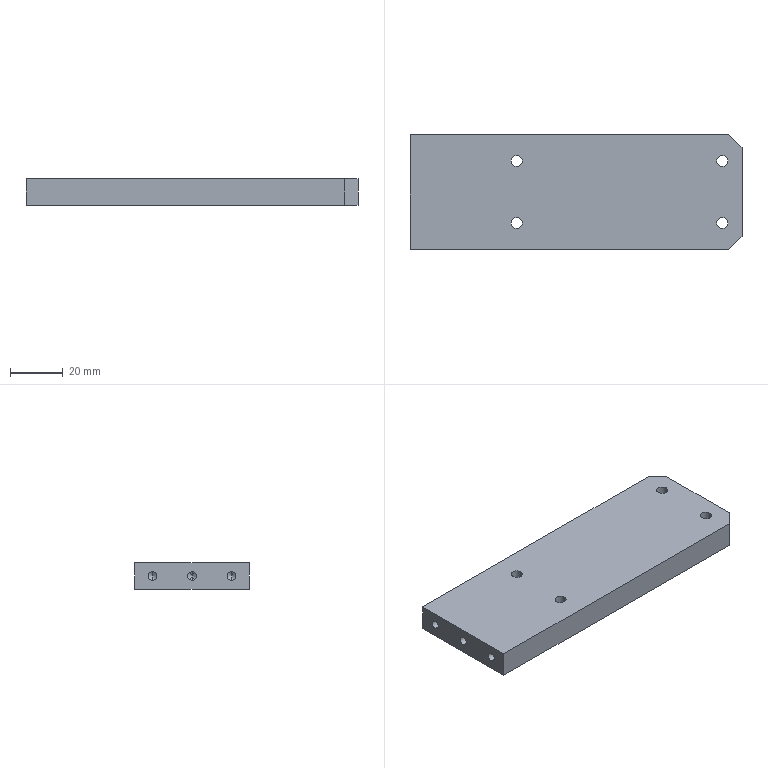Part | SolidWorks | features HoleWzd 2, Chamfer 1, Extrusion 1 | 1 solid | 28 faces | box 126 x 43.6 x 10 mm | volume 53864 mm3 | cylinder 14 | plane 8 | cone 6 | commonest cylinder face diameters 4.2 x8 3.3 x6
STEP:
#1=CARTESIAN_POINT('',(42.6,33.55,0.));
#2=VERTEX_POINT('',#1);
#3=CARTESIAN_POINT('',(38.4,33.55,0.));
#4=VERTEX_POINT('',#3);
#5=CARTESIAN_POINT('',(40.5,33.55,0.));
#6=DIRECTION('',(0.,0.,-1.));
#7=DIRECTION('',(-1.,0.,0.));
#8=AXIS2_PLACEMENT_3D('',#5,#6,#7);
#9=CIRCLE('',#8,2.1);
#10=EDGE_CURVE('',#2,#4,#9,.T.);
#11=ORIENTED_EDGE('',*,*,#10,.F.);
#12=CARTESIAN_POINT('',(42.6,33.55,-10.));
#13=VERTEX_POINT('',#12);
#14=CARTESIAN_POINT('',(42.6,33.55,-10.));
#15=DIRECTION('',(0.,0.,-1.));
#16=VECTOR('',#15,1000.);
#17=LINE('',#14,#16);
#18=EDGE_CURVE('',#2,#13,#17,.T.);
#19=ORIENTED_EDGE('',*,*,#18,.T.);
#20=CARTESIAN_POINT('',(38.4,33.55,-10.));
#21=VERTEX_POINT('',#20);
#22=CARTESIAN_POINT('',(40.5,33.55,-10.));
#23=DIRECTION('',(0.,0.,-1.));
#24=DIRECTION('',(-1.,0.,0.));
#25=AXIS2_PLACEMENT_3D('',#22,#23,#24);
#26=CIRCLE('',#25,2.1);
#27=EDGE_CURVE('',#13,#21,#26,.T.);
#28=ORIENTED_EDGE('',*,*,#27,.T.);
#29=CARTESIAN_POINT('',(38.4,33.55,-10.));
#30=DIRECTION('',(0.,0.,-1.));
#31=VECTOR('',#30,1000.);
#32=LINE('',#29,#31);
#33=EDGE_CURVE('',#4,#21,#32,.T.);
#34=ORIENTED_EDGE('',*,*,#33,.F.);
#35=EDGE_LOOP('',(#11,#19,#28,#34));
#36=FACE_OUTER_BOUND('',#35,.T.);
#37=CARTESIAN_POINT('',(40.5,33.55,-10.));
#38=DIRECTION('',(0.,0.,-1.));
#39=DIRECTION('',(-1.,0.,0.));
#40=AXIS2_PLACEMENT_3D('',#37,#38,#39);
#41=CYLINDRICAL_SURFACE('',#40,2.1);
#42=ADVANCED_FACE('',(#36),#41,.F.);
#43=CARTESIAN_POINT('',(42.6,10.05,0.));
#44=VERTEX_POINT('',#43);
#45=CARTESIAN_POINT('',(38.4,10.05,0.));
#46=VERTEX_POINT('',#45);
#47=CARTESIAN_POINT('',(40.5,10.05,0.));
#48=DIRECTION('',(0.,0.,-1.));
#49=DIRECTION('',(-1.,0.,0.));
#50=AXIS2_PLACEMENT_3D('',#47,#48,#49);
#51=CIRCLE('',#50,2.1);
#52=EDGE_CURVE('',#44,#46,#51,.T.);
#53=ORIENTED_EDGE('',*,*,#52,.F.);
#54=CARTESIAN_POINT('',(42.6,10.05,-10.));
#55=VERTEX_POINT('',#54);
#56=CARTESIAN_POINT('',(42.6,10.05,-10.));
#57=DIRECTION('',(0.,0.,-1.));
#58=VECTOR('',#57,1000.);
#59=LINE('',#56,#58);
#60=EDGE_CURVE('',#44,#55,#59,.T.);
#61=ORIENTED_EDGE('',*,*,#60,.T.);
#62=CARTESIAN_POINT('',(38.4,10.05,-10.));
#63=VERTEX_POINT('',#62);
#64=CARTESIAN_POINT('',(40.5,10.05,-10.));
#65=DIRECTION('',(0.,0.,-1.));
#66=DIRECTION('',(-1.,0.,0.));
#67=AXIS2_PLACEMENT_3D('',#64,#65,#66);
#68=CIRCLE('',#67,2.1);
#69=EDGE_CURVE('',#55,#63,#68,.T.);
#70=ORIENTED_EDGE('',*,*,#69,.T.);
#71=CARTESIAN_POINT('',(38.4,10.05,-10.));
#72=DIRECTION('',(0.,0.,-1.));
#73=VECTOR('',#72,1000.);
#74=LINE('',#71,#73);
#75=EDGE_CURVE('',#46,#63,#74,.T.);
#76=ORIENTED_EDGE('',*,*,#75,.F.);
#77=EDGE_LOOP('',(#53,#61,#70,#76));
#78=FACE_OUTER_BOUND('',#77,.T.);
#79=CARTESIAN_POINT('',(40.5,10.05,-10.));
#80=DIRECTION('',(0.,0.,-1.));
#81=DIRECTION('',(-1.,0.,0.));
#82=AXIS2_PLACEMENT_3D('',#79,#80,#81);
#83=CYLINDRICAL_SURFACE('',#82,2.1);
#84=ADVANCED_FACE('',(#78),#83,.F.);
#85=CARTESIAN_POINT('',(120.6,33.55,0.));
#86=VERTEX_POINT('',#85);
#87=CARTESIAN_POINT('',(116.4,33.55,0.));
#88=VERTEX_POINT('',#87);
#89=CARTESIAN_POINT('',(118.5,33.55,0.));
#90=DIRECTION('',(0.,0.,-1.));
#91=DIRECTION('',(-1.,0.,0.));
#92=AXIS2_PLACEMENT_3D('',#89,#90,#91);
#93=CIRCLE('',#92,2.1);
#94=EDGE_CURVE('',#86,#88,#93,.T.);
#95=ORIENTED_EDGE('',*,*,#94,.F.);
#96=CARTESIAN_POINT('',(120.6,33.55,-10.));
#97=VERTEX_POINT('',#96);
#98=CARTESIAN_POINT('',(120.6,33.55,-10.));
#99=DIRECTION('',(0.,0.,-1.));
#100=VECTOR('',#99,1000.);
#101=LINE('',#98,#100);
#102=EDGE_CURVE('',#86,#97,#101,.T.);
#103=ORIENTED_EDGE('',*,*,#102,.T.);
#104=CARTESIAN_POINT('',(116.4,33.55,-10.));
#105=VERTEX_POINT('',#104);
#106=CARTESIAN_POINT('',(118.5,33.55,-10.));
#107=DIRECTION('',(0.,0.,-1.));
#108=DIRECTION('',(-1.,0.,0.));
#109=AXIS2_PLACEMENT_3D('',#106,#107,#108);
#110=CIRCLE('',#109,2.1);
#111=EDGE_CURVE('',#97,#105,#110,.T.);
#112=ORIENTED_EDGE('',*,*,#111,.T.);
#113=CARTESIAN_POINT('',(116.4,33.55,-10.));
#114=DIRECTION('',(0.,0.,-1.));
#115=VECTOR('',#114,1000.);
#116=LINE('',#113,#115);
#117=EDGE_CURVE('',#88,#105,#116,.T.);
#118=ORIENTED_EDGE('',*,*,#117,.F.);
#119=EDGE_LOOP('',(#95,#103,#112,#118));
#120=FACE_OUTER_BOUND('',#119,.T.);
#121=CARTESIAN_POINT('',(118.5,33.55,-10.));
#122=DIRECTION('',(0.,0.,-1.));
#123=DIRECTION('',(-1.,0.,0.));
#124=AXIS2_PLACEMENT_3D('',#121,#122,#123);
#125=CYLINDRICAL_SURFACE('',#124,2.1);
#126=ADVANCED_FACE('',(#120),#125,.F.);
#127=CARTESIAN_POINT('',(120.6,10.05,0.));
#128=VERTEX_POINT('',#127);
#129=CARTESIAN_POINT('',(116.4,10.05,0.));
#130=VERTEX_POINT('',#129);
#131=CARTESIAN_POINT('',(118.5,10.05,0.));
#132=DIRECTION('',(0.,0.,-1.));
#133=DIRECTION('',(-1.,0.,0.));
#134=AXIS2_PLACEMENT_3D('',#131,#132,#133);
#135=CIRCLE('',#134,2.1);
#136=EDGE_CURVE('',#128,#130,#135,.T.);
#137=ORIENTED_EDGE('',*,*,#136,.F.);
#138=CARTESIAN_POINT('',(120.6,10.05,-10.));
#139=VERTEX_POINT('',#138);
#140=CARTESIAN_POINT('',(120.6,10.05,-10.));
#141=DIRECTION('',(0.,0.,-1.));
#142=VECTOR('',#141,1000.);
#143=LINE('',#140,#142);
#144=EDGE_CURVE('',#128,#139,#143,.T.);
#145=ORIENTED_EDGE('',*,*,#144,.T.);
#146=CARTESIAN_POINT('',(116.4,10.05,-10.));
#147=VERTEX_POINT('',#146);
#148=CARTESIAN_POINT('',(118.5,10.05,-10.));
#149=DIRECTION('',(0.,0.,-1.));
#150=DIRECTION('',(-1.,0.,0.));
#151=AXIS2_PLACEMENT_3D('',#148,#149,#150);
#152=CIRCLE('',#151,2.1);
#153=EDGE_CURVE('',#139,#147,#152,.T.);
#154=ORIENTED_EDGE('',*,*,#153,.T.);
#155=CARTESIAN_POINT('',(116.4,10.05,-10.));
#156=DIRECTION('',(0.,0.,-1.));
#157=VECTOR('',#156,1000.);
#158=LINE('',#155,#157);
#159=EDGE_CURVE('',#130,#147,#158,.T.);
#160=ORIENTED_EDGE('',*,*,#159,.F.);
#161=EDGE_LOOP('',(#137,#145,#154,#160));
#162=FACE_OUTER_BOUND('',#161,.T.);
#163=CARTESIAN_POINT('',(118.5,10.05,-10.));
#164=DIRECTION('',(0.,0.,-1.));
#165=DIRECTION('',(-1.,0.,0.));
#166=AXIS2_PLACEMENT_3D('',#163,#164,#165);
#167=CYLINDRICAL_SURFACE('',#166,2.1);
#168=ADVANCED_FACE('',(#162),#167,.F.);
#169=CARTESIAN_POINT('',(10.1,36.8,-6.65));
#170=VERTEX_POINT('',#169);
#171=CARTESIAN_POINT('',(10.1,36.8,-3.35));
#172=VERTEX_POINT('',#171);
#173=CARTESIAN_POINT('',(10.1,36.8,-5.));
#174=DIRECTION('',(-1.,0.,0.));
#175=DIRECTION('',(0.,0.,1.));
#176=AXIS2_PLACEMENT_3D('',#173,#174,#175);
#177=CIRCLE('',#176,1.65);
#178=EDGE_CURVE('',#170,#172,#177,.T.);
#179=ORIENTED_EDGE('',*,*,#178,.F.);
#180=CARTESIAN_POINT('',(0.,36.8,-6.65));
#181=VERTEX_POINT('',#180);
#182=CARTESIAN_POINT('',(0.,36.8,-6.65));
#183=DIRECTION('',(-1.,0.,0.));
#184=VECTOR('',#183,1000.);
#185=LINE('',#182,#184);
#186=EDGE_CURVE('',#170,#181,#185,.T.);
#187=ORIENTED_EDGE('',*,*,#186,.T.);
#188=CARTESIAN_POINT('',(0.,36.8,-3.35));
#189=VERTEX_POINT('',#188);
#190=CARTESIAN_POINT('',(0.,36.8,-5.));
#191=DIRECTION('',(-1.,0.,0.));
#192=DIRECTION('',(0.,0.,1.));
#193=AXIS2_PLACEMENT_3D('',#190,#191,#192);
#194=CIRCLE('',#193,1.65);
#195=EDGE_CURVE('',#181,#189,#194,.T.);
#196=ORIENTED_EDGE('',*,*,#195,.T.);
#197=CARTESIAN_POINT('',(0.,36.8,-3.35));
#198=DIRECTION('',(-1.,0.,0.));
#199=VECTOR('',#198,1000.);
#200=LINE('',#197,#199);
#201=EDGE_CURVE('',#172,#189,#200,.T.);
#202=ORIENTED_EDGE('',*,*,#201,.F.);
#203=EDGE_LOOP('',(#179,#187,#196,#202));
#204=FACE_OUTER_BOUND('',#203,.T.);
#205=CARTESIAN_POINT('',(0.,36.8,-5.));
#206=DIRECTION('',(-1.,0.,0.));
#207=DIRECTION('',(0.,0.,1.));
#208=AXIS2_PLACEMENT_3D('',#205,#206,#207);
#209=CYLINDRICAL_SURFACE('',#208,1.65);
#210=ADVANCED_FACE('',(#204),#209,.F.);
#211=CARTESIAN_POINT('',(11.091,36.8,-5.));
#212=VERTEX_POINT('',#211);
#213=CARTESIAN_POINT('',(10.1,36.8,-3.35));
#214=DIRECTION('',(-0.515,0.,0.8572));
#215=VECTOR('',#214,1000.);
#216=LINE('',#213,#215);
#217=EDGE_CURVE('',#212,#172,#216,.T.);
#218=ORIENTED_EDGE('',*,*,#217,.F.);
#219=CARTESIAN_POINT('',(10.1,36.8,-6.65));
#220=DIRECTION('',(-0.515,0.,-0.8572));
#221=VECTOR('',#220,1000.);
#222=LINE('',#219,#221);
#223=EDGE_CURVE('',#212,#170,#222,.T.);
#224=ORIENTED_EDGE('',*,*,#223,.T.);
#225=ORIENTED_EDGE('',*,*,#178,.T.);
#226=EDGE_LOOP('',(#218,#224,#225));
#227=FACE_OUTER_BOUND('',#226,.T.);
#228=CARTESIAN_POINT('',(10.1,36.8,-5.));
#229=DIRECTION('',(-1.,0.,0.));
#230=DIRECTION('',(0.,0.,1.));
#231=AXIS2_PLACEMENT_3D('',#228,#229,#230);
#232=CONICAL_SURFACE('',#231,1.65,1.03);
#233=ADVANCED_FACE('',(#227),#232,.F.);
#234=CARTESIAN_POINT('',(10.1,21.783,-6.65));
#235=VERTEX_POINT('',#234);
#236=CARTESIAN_POINT('',(10.1,21.783,-3.35));
#237=VERTEX_POINT('',#236);
#238=CARTESIAN_POINT('',(10.1,21.783,-5.));
#239=DIRECTION('',(-1.,0.,0.));
#240=DIRECTION('',(0.,0.,1.));
#241=AXIS2_PLACEMENT_3D('',#238,#239,#240);
#242=CIRCLE('',#241,1.65);
#243=EDGE_CURVE('',#235,#237,#242,.T.);
#244=ORIENTED_EDGE('',*,*,#243,.F.);
#245=CARTESIAN_POINT('',(0.,21.783,-6.65));
#246=VERTEX_POINT('',#245);
#247=CARTESIAN_POINT('',(0.,21.783,-6.65));
#248=DIRECTION('',(-1.,0.,0.));
#249=VECTOR('',#248,1000.);
#250=LINE('',#247,#249);
#251=EDGE_CURVE('',#235,#246,#250,.T.);
#252=ORIENTED_EDGE('',*,*,#251,.T.);
#253=CARTESIAN_POINT('',(0.,21.783,-3.35));
#254=VERTEX_POINT('',#253);
#255=CARTESIAN_POINT('',(0.,21.783,-5.));
#256=DIRECTION('',(-1.,0.,0.));
#257=DIRECTION('',(0.,0.,1.));
#258=AXIS2_PLACEMENT_3D('',#255,#256,#257);
#259=CIRCLE('',#258,1.65);
#260=EDGE_CURVE('',#246,#254,#259,.T.);
#261=ORIENTED_EDGE('',*,*,#260,.T.);
#262=CARTESIAN_POINT('',(0.,21.783,-3.35));
#263=DIRECTION('',(-1.,0.,0.));
#264=VECTOR('',#263,1000.);
#265=LINE('',#262,#264);
#266=EDGE_CURVE('',#237,#254,#265,.T.);
#267=ORIENTED_EDGE('',*,*,#266,.F.);
#268=EDGE_LOOP('',(#244,#252,#261,#267));
#269=FACE_OUTER_BOUND('',#268,.T.);
#270=CARTESIAN_POINT('',(0.,21.783,-5.));
#271=DIRECTION('',(-1.,0.,0.));
#272=DIRECTION('',(0.,0.,1.));
#273=AXIS2_PLACEMENT_3D('',#270,#271,#272);
#274=CYLINDRICAL_SURFACE('',#273,1.65);
#275=ADVANCED_FACE('',(#269),#274,.F.);
#276=CARTESIAN_POINT('',(11.091,21.783,-5.));
#277=VERTEX_POINT('',#276);
#278=CARTESIAN_POINT('',(10.1,21.783,-3.35));
#279=DIRECTION('',(-0.515,0.,0.8572));
#280=VECTOR('',#279,1000.);
#281=LINE('',#278,#280);
#282=EDGE_CURVE('',#277,#237,#281,.T.);
#283=ORIENTED_EDGE('',*,*,#282,.F.);
#284=CARTESIAN_POINT('',(10.1,21.783,-6.65));
#285=DIRECTION('',(-0.515,0.,-0.8572));
#286=VECTOR('',#285,1000.);
#287=LINE('',#284,#286);
#288=EDGE_CURVE('',#277,#235,#287,.T.);
#289=ORIENTED_EDGE('',*,*,#288,.T.);
#290=ORIENTED_EDGE('',*,*,#243,.T.);
#291=EDGE_LOOP('',(#283,#289,#290));
#292=FACE_OUTER_BOUND('',#291,.T.);
#293=CARTESIAN_POINT('',(10.1,21.783,-5.));
#294=DIRECTION('',(-1.,0.,0.));
#295=DIRECTION('',(0.,0.,1.));
#296=AXIS2_PLACEMENT_3D('',#293,#294,#295);
#297=CONICAL_SURFACE('',#296,1.65,1.03);
#298=ADVANCED_FACE('',(#292),#297,.F.);
#299=CARTESIAN_POINT('',(10.1,6.8,-6.65));
#300=VERTEX_POINT('',#299);
#301=CARTESIAN_POINT('',(10.1,6.8,-3.35));
#302=VERTEX_POINT('',#301);
#303=CARTESIAN_POINT('',(10.1,6.8,-5.));
#304=DIRECTION('',(-1.,0.,0.));
#305=DIRECTION('',(0.,0.,1.));
#306=AXIS2_PLACEMENT_3D('',#303,#304,#305);
#307=CIRCLE('',#306,1.65);
#308=EDGE_CURVE('',#300,#302,#307,.T.);
#309=ORIENTED_EDGE('',*,*,#308,.F.);
#310=CARTESIAN_POINT('',(0.,6.8,-6.65));
#311=VERTEX_POINT('',#310);
#312=CARTESIAN_POINT('',(0.,6.8,-6.65));
#313=DIRECTION('',(-1.,0.,0.));
#314=VECTOR('',#313,1000.);
#315=LINE('',#312,#314);
#316=EDGE_CURVE('',#300,#311,#315,.T.);
#317=ORIENTED_EDGE('',*,*,#316,.T.);
#318=CARTESIAN_POINT('',(0.,6.8,-3.35));
#319=VERTEX_POINT('',#318);
#320=CARTESIAN_POINT('',(0.,6.8,-5.));
#321=DIRECTION('',(-1.,0.,0.));
#322=DIRECTION('',(0.,0.,1.));
#323=AXIS2_PLACEMENT_3D('',#320,#321,#322);
#324=CIRCLE('',#323,1.65);
#325=EDGE_CURVE('',#311,#319,#324,.T.);
#326=ORIENTED_EDGE('',*,*,#325,.T.);
#327=CARTESIAN_POINT('',(0.,6.8,-3.35));
#328=DIRECTION('',(-1.,0.,0.));
#329=VECTOR('',#328,1000.);
#330=LINE('',#327,#329);
#331=EDGE_CURVE('',#302,#319,#330,.T.);
#332=ORIENTED_EDGE('',*,*,#331,.F.);
#333=EDGE_LOOP('',(#309,#317,#326,#332));
#334=FACE_OUTER_BOUND('',#333,.T.);
#335=CARTESIAN_POINT('',(0.,6.8,-5.));
#336=DIRECTION('',(-1.,0.,0.));
#337=DIRECTION('',(0.,0.,1.));
#338=AXIS2_PLACEMENT_3D('',#335,#336,#337);
#339=CYLINDRICAL_SURFACE('',#338,1.65);
#340=ADVANCED_FACE('',(#334),#339,.F.);
#341=CARTESIAN_POINT('',(11.091,6.8,-5.));
#342=VERTEX_POINT('',#341);
#343=CARTESIAN_POINT('',(10.1,6.8,-3.35));
#344=DIRECTION('',(-0.515,0.,0.8572));
#345=VECTOR('',#344,1000.);
#346=LINE('',#343,#345);
#347=EDGE_CURVE('',#342,#302,#346,.T.);
#348=ORIENTED_EDGE('',*,*,#347,.F.);
#349=CARTESIAN_POINT('',(10.1,6.8,-6.65));
#350=DIRECTION('',(-0.515,0.,-0.8572));
#351=VECTOR('',#350,1000.);
#352=LINE('',#349,#351);
#353=EDGE_CURVE('',#342,#300,#352,.T.);
#354=ORIENTED_EDGE('',*,*,#353,.T.);
#355=ORIENTED_EDGE('',*,*,#308,.T.);
#356=EDGE_LOOP('',(#348,#354,#355));
#357=FACE_OUTER_BOUND('',#356,.T.);
#358=CARTESIAN_POINT('',(10.1,6.8,-5.));
#359=DIRECTION('',(-1.,0.,0.));
#360=DIRECTION('',(0.,0.,1.));
#361=AXIS2_PLACEMENT_3D('',#358,#359,#360);
#362=CONICAL_SURFACE('',#361,1.65,1.03);
#363=ADVANCED_FACE('',(#357),#362,.F.);
#364=CARTESIAN_POINT('',(0.,36.8,-5.));
#365=DIRECTION('',(-1.,0.,0.));
#366=DIRECTION('',(0.,0.,1.));
#367=AXIS2_PLACEMENT_3D('',#364,#365,#366);
#368=CIRCLE('',#367,1.65);
#369=EDGE_CURVE('',#189,#181,#368,.T.);
#370=ORIENTED_EDGE('',*,*,#369,.F.);
#371=ORIENTED_EDGE('',*,*,#195,.F.);
#372=EDGE_LOOP('',(#370,#371));
#373=FACE_BOUND('',#372,.T.);
#374=CARTESIAN_POINT('',(0.,21.783,-5.));
#375=DIRECTION('',(-1.,0.,0.));
#376=DIRECTION('',(0.,0.,1.));
#377=AXIS2_PLACEMENT_3D('',#374,#375,#376);
#378=CIRCLE('',#377,1.65);
#379=EDGE_CURVE('',#254,#246,#378,.T.);
#380=ORIENTED_EDGE('',*,*,#379,.F.);
#381=ORIENTED_EDGE('',*,*,#260,.F.);
#382=EDGE_LOOP('',(#380,#381));
#383=FACE_BOUND('',#382,.T.);
#384=CARTESIAN_POINT('',(0.,6.8,-5.));
#385=DIRECTION('',(-1.,0.,0.));
#386=DIRECTION('',(0.,0.,1.));
#387=AXIS2_PLACEMENT_3D('',#384,#385,#386);
#388=CIRCLE('',#387,1.65);
#389=EDGE_CURVE('',#319,#311,#388,.T.);
#390=ORIENTED_EDGE('',*,*,#389,.F.);
#391=ORIENTED_EDGE('',*,*,#325,.F.);
#392=EDGE_LOOP('',(#390,#391));
#393=FACE_BOUND('',#392,.T.);
#394=CARTESIAN_POINT('',(0.,0.,-10.));
#395=VERTEX_POINT('',#394);
#396=CARTESIAN_POINT('',(0.,0.,0.));
#397=VERTEX_POINT('',#396);
#398=CARTESIAN_POINT('',(0.,0.,0.));
#399=DIRECTION('',(0.,0.,1.));
#400=VECTOR('',#399,1000.);
#401=LINE('',#398,#400);
#402=EDGE_CURVE('',#395,#397,#401,.T.);
#403=ORIENTED_EDGE('',*,*,#402,.T.);
#404=CARTESIAN_POINT('',(0.,43.6,0.));
#405=VERTEX_POINT('',#404);
#406=CARTESIAN_POINT('',(0.,43.6,0.));
#407=DIRECTION('',(0.,-1.,0.));
#408=VECTOR('',#407,1000.);
#409=LINE('',#406,#408);
#410=EDGE_CURVE('',#405,#397,#409,.T.);
#411=ORIENTED_EDGE('',*,*,#410,.F.);
#412=CARTESIAN_POINT('',(0.,43.6,-10.));
#413=VERTEX_POINT('',#412);
#414=CARTESIAN_POINT('',(0.,43.6,0.));
#415=DIRECTION('',(0.,0.,1.));
#416=VECTOR('',#415,1000.);
#417=LINE('',#414,#416);
#418=EDGE_CURVE('',#413,#405,#417,.T.);
#419=ORIENTED_EDGE('',*,*,#418,.F.);
#420=CARTESIAN_POINT('',(0.,43.6,-10.));
#421=DIRECTION('',(0.,-1.,0.));
#422=VECTOR('',#421,1000.);
#423=LINE('',#420,#422);
#424=EDGE_CURVE('',#413,#395,#423,.T.);
#425=ORIENTED_EDGE('',*,*,#424,.T.);
#426=EDGE_LOOP('',(#403,#411,#419,#425));
#427=FACE_OUTER_BOUND('',#426,.T.);
#428=CARTESIAN_POINT('',(0.,43.6,0.));
#429=DIRECTION('',(1.,0.,0.));
#430=DIRECTION('',(0.,0.,-1.));
#431=AXIS2_PLACEMENT_3D('',#428,#429,#430);
#432=PLANE('',#431);
#433=ADVANCED_FACE('',(#373,#383,#393,#427),#432,.F.);
#434=CARTESIAN_POINT('',(40.5,33.55,0.));
#435=DIRECTION('',(0.,0.,-1.));
#436=DIRECTION('',(-1.,0.,0.));
#437=AXIS2_PLACEMENT_3D('',#434,#435,#436);
#438=CIRCLE('',#437,2.1);
#439=EDGE_CURVE('',#4,#2,#438,.T.);
#440=ORIENTED_EDGE('',*,*,#439,.T.);
#441=ORIENTED_EDGE('',*,*,#10,.T.);
#442=EDGE_LOOP('',(#440,#441));
#443=FACE_BOUND('',#442,.T.);
#444=CARTESIAN_POINT('',(40.5,10.05,0.));
#445=DIRECTION('',(0.,0.,-1.));
#446=DIRECTION('',(-1.,0.,0.));
#447=AXIS2_PLACEMENT_3D('',#444,#445,#446);
#448=CIRCLE('',#447,2.1);
#449=EDGE_CURVE('',#46,#44,#448,.T.);
#450=ORIENTED_EDGE('',*,*,#449,.T.);
#451=ORIENTED_EDGE('',*,*,#52,.T.);
#452=EDGE_LOOP('',(#450,#451));
#453=FACE_BOUND('',#452,.T.);
#454=CARTESIAN_POINT('',(118.5,33.55,0.));
#455=DIRECTION('',(0.,0.,-1.));
#456=DIRECTION('',(-1.,0.,0.));
#457=AXIS2_PLACEMENT_3D('',#454,#455,#456);
#458=CIRCLE('',#457,2.1);
#459=EDGE_CURVE('',#88,#86,#458,.T.);
#460=ORIENTED_EDGE('',*,*,#459,.T.);
#461=ORIENTED_EDGE('',*,*,#94,.T.);
#462=EDGE_LOOP('',(#460,#461));
#463=FACE_BOUND('',#462,.T.);
#464=CARTESIAN_POINT('',(118.5,10.05,0.));
#465=DIRECTION('',(0.,0.,-1.));
#466=DIRECTION('',(-1.,0.,0.));
#467=AXIS2_PLACEMENT_3D('',#464,#465,#466);
#468=CIRCLE('',#467,2.1);
#469=EDGE_CURVE('',#130,#128,#468,.T.);
#470=ORIENTED_EDGE('',*,*,#469,.T.);
#471=ORIENTED_EDGE('',*,*,#136,.T.);
#472=EDGE_LOOP('',(#470,#471));
#473=FACE_BOUND('',#472,.T.);
#474=CARTESIAN_POINT('',(121.,0.,0.));
#475=VERTEX_POINT('',#474);
#476=CARTESIAN_POINT('',(0.,0.,0.));
#477=DIRECTION('',(1.,0.,0.));
#478=VECTOR('',#477,1000.);
#479=LINE('',#476,#478);
#480=EDGE_CURVE('',#397,#475,#479,.T.);
#481=ORIENTED_EDGE('',*,*,#480,.T.);
#482=CARTESIAN_POINT('',(126.,5.,0.));
#483=VERTEX_POINT('',#482);
#484=CARTESIAN_POINT('',(126.,5.,0.));
#485=DIRECTION('',(0.7071,0.7071,0.));
#486=VECTOR('',#485,1000.);
#487=LINE('',#484,#486);
#488=EDGE_CURVE('',#475,#483,#487,.T.);
#489=ORIENTED_EDGE('',*,*,#488,.T.);
#490=CARTESIAN_POINT('',(126.,38.6,0.));
#491=VERTEX_POINT('',#490);
#492=CARTESIAN_POINT('',(126.,43.6,0.));
#493=DIRECTION('',(0.,-1.,0.));
#494=VECTOR('',#493,1000.);
#495=LINE('',#492,#494);
#496=EDGE_CURVE('',#491,#483,#495,.T.);
#497=ORIENTED_EDGE('',*,*,#496,.F.);
#498=CARTESIAN_POINT('',(121.,43.6,0.));
#499=VERTEX_POINT('',#498);
#500=CARTESIAN_POINT('',(121.,43.6,0.));
#501=DIRECTION('',(-0.7071,0.7071,0.));
#502=VECTOR('',#501,1000.);
#503=LINE('',#500,#502);
#504=EDGE_CURVE('',#491,#499,#503,.T.);
#505=ORIENTED_EDGE('',*,*,#504,.T.);
#506=CARTESIAN_POINT('',(0.,43.6,0.));
#507=DIRECTION('',(1.,0.,0.));
#508=VECTOR('',#507,1000.);
#509=LINE('',#506,#508);
#510=EDGE_CURVE('',#405,#499,#509,.T.);
#511=ORIENTED_EDGE('',*,*,#510,.F.);
#512=ORIENTED_EDGE('',*,*,#410,.T.);
#513=EDGE_LOOP('',(#481,#489,#497,#505,#511,#512));
#514=FACE_OUTER_BOUND('',#513,.T.);
#515=CARTESIAN_POINT('',(0.,43.6,0.));
#516=DIRECTION('',(0.,0.,-1.));
#517=DIRECTION('',(-1.,0.,0.));
#518=AXIS2_PLACEMENT_3D('',#515,#516,#517);
#519=PLANE('',#518);
#520=ADVANCED_FACE('',(#443,#453,#463,#473,#514),#519,.F.);
#521=ORIENTED_EDGE('',*,*,#496,.T.);
#522=CARTESIAN_POINT('',(126.,5.,-10.));
#523=VERTEX_POINT('',#522);
#524=CARTESIAN_POINT('',(126.,5.,-10.));
#525=DIRECTION('',(0.,0.,-1.));
#526=VECTOR('',#525,1000.);
#527=LINE('',#524,#526);
#528=EDGE_CURVE('',#483,#523,#527,.T.);
#529=ORIENTED_EDGE('',*,*,#528,.T.);
#530=CARTESIAN_POINT('',(126.,38.6,-10.));
#531=VERTEX_POINT('',#530);
#532=CARTESIAN_POINT('',(126.,43.6,-10.));
#533=DIRECTION('',(0.,-1.,0.));
#534=VECTOR('',#533,1000.);
#535=LINE('',#532,#534);
#536=EDGE_CURVE('',#531,#523,#535,.T.);
#537=ORIENTED_EDGE('',*,*,#536,.F.);
#538=CARTESIAN_POINT('',(126.,38.6,0.));
#539=DIRECTION('',(0.,0.,1.));
#540=VECTOR('',#539,1000.);
#541=LINE('',#538,#540);
#542=EDGE_CURVE('',#531,#491,#541,.T.);
#543=ORIENTED_EDGE('',*,*,#542,.T.);
#544=EDGE_LOOP('',(#521,#529,#537,#543));
#545=FACE_OUTER_BOUND('',#544,.T.);
#546=CARTESIAN_POINT('',(126.,43.6,0.));
#547=DIRECTION('',(-1.,0.,0.));
#548=DIRECTION('',(0.,0.,1.));
#549=AXIS2_PLACEMENT_3D('',#546,#547,#548);
#550=PLANE('',#549);
#551=ADVANCED_FACE('',(#545),#550,.F.);
#552=CARTESIAN_POINT('',(40.5,33.55,-10.));
#553=DIRECTION('',(0.,0.,-1.));
#554=DIRECTION('',(-1.,0.,0.));
#555=AXIS2_PLACEMENT_3D('',#552,#553,#554);
#556=CIRCLE('',#555,2.1);
#557=EDGE_CURVE('',#21,#13,#556,.T.);
#558=ORIENTED_EDGE('',*,*,#557,.F.);
#559=ORIENTED_EDGE('',*,*,#27,.F.);
#560=EDGE_LOOP('',(#558,#559));
#561=FACE_BOUND('',#560,.T.);
#562=CARTESIAN_POINT('',(40.5,10.05,-10.));
#563=DIRECTION('',(0.,0.,-1.));
#564=DIRECTION('',(-1.,0.,0.));
#565=AXIS2_PLACEMENT_3D('',#562,#563,#564);
#566=CIRCLE('',#565,2.1);
#567=EDGE_CURVE('',#63,#55,#566,.T.);
#568=ORIENTED_EDGE('',*,*,#567,.F.);
#569=ORIENTED_EDGE('',*,*,#69,.F.);
#570=EDGE_LOOP('',(#568,#569));
#571=FACE_BOUND('',#570,.T.);
#572=CARTESIAN_POINT('',(118.5,33.55,-10.));
#573=DIRECTION('',(0.,0.,-1.));
#574=DIRECTION('',(-1.,0.,0.));
#575=AXIS2_PLACEMENT_3D('',#572,#573,#574);
#576=CIRCLE('',#575,2.1);
#577=EDGE_CURVE('',#105,#97,#576,.T.);
#578=ORIENTED_EDGE('',*,*,#577,.F.);
#579=ORIENTED_EDGE('',*,*,#111,.F.);
#580=EDGE_LOOP('',(#578,#579));
#581=FACE_BOUND('',#580,.T.);
#582=CARTESIAN_POINT('',(118.5,10.05,-10.));
#583=DIRECTION('',(0.,0.,-1.));
#584=DIRECTION('',(-1.,0.,0.));
#585=AXIS2_PLACEMENT_3D('',#582,#583,#584);
#586=CIRCLE('',#585,2.1);
#587=EDGE_CURVE('',#147,#139,#586,.T.);
#588=ORIENTED_EDGE('',*,*,#587,.F.);
#589=ORIENTED_EDGE('',*,*,#153,.F.);
#590=EDGE_LOOP('',(#588,#589));
#591=FACE_BOUND('',#590,.T.);
#592=ORIENTED_EDGE('',*,*,#536,.T.);
#593=CARTESIAN_POINT('',(121.,0.,-10.));
#594=VERTEX_POINT('',#593);
#595=CARTESIAN_POINT('',(126.,5.,-10.));
#596=DIRECTION('',(-0.7071,-0.7071,0.));
#597=VECTOR('',#596,1000.);
#598=LINE('',#595,#597);
#599=EDGE_CURVE('',#523,#594,#598,.T.);
#600=ORIENTED_EDGE('',*,*,#599,.T.);
#601=CARTESIAN_POINT('',(0.,0.,-10.));
#602=DIRECTION('',(-1.,0.,0.));
#603=VECTOR('',#602,1000.);
#604=LINE('',#601,#603);
#605=EDGE_CURVE('',#594,#395,#604,.T.);
#606=ORIENTED_EDGE('',*,*,#605,.T.);
#607=ORIENTED_EDGE('',*,*,#424,.F.);
#608=CARTESIAN_POINT('',(121.,43.6,-10.));
#609=VERTEX_POINT('',#608);
#610=CARTESIAN_POINT('',(0.,43.6,-10.));
#611=DIRECTION('',(-1.,0.,0.));
#612=VECTOR('',#611,1000.);
#613=LINE('',#610,#612);
#614=EDGE_CURVE('',#609,#413,#613,.T.);
#615=ORIENTED_EDGE('',*,*,#614,.F.);
#616=CARTESIAN_POINT('',(121.,43.6,-10.));
#617=DIRECTION('',(0.7071,-0.7071,0.));
#618=VECTOR('',#617,1000.);
#619=LINE('',#616,#618);
#620=EDGE_CURVE('',#609,#531,#619,.T.);
#621=ORIENTED_EDGE('',*,*,#620,.T.);
#622=EDGE_LOOP('',(#592,#600,#606,#607,#615,#621));
#623=FACE_OUTER_BOUND('',#622,.T.);
#624=CARTESIAN_POINT('',(0.,43.6,-10.));
#625=DIRECTION('',(0.,0.,1.));
#626=DIRECTION('',(1.,0.,0.));
#627=AXIS2_PLACEMENT_3D('',#624,#625,#626);
#628=PLANE('',#627);
#629=ADVANCED_FACE('',(#561,#571,#581,#591,#623),#628,.F.);
#630=ORIENTED_EDGE('',*,*,#510,.T.);
#631=CARTESIAN_POINT('',(121.,43.6,0.));
#632=DIRECTION('',(0.,0.,-1.));
#633=VECTOR('',#632,1000.);
#634=LINE('',#631,#633);
#635=EDGE_CURVE('',#499,#609,#634,.T.);
#636=ORIENTED_EDGE('',*,*,#635,.T.);
#637=ORIENTED_EDGE('',*,*,#614,.T.);
#638=ORIENTED_EDGE('',*,*,#418,.T.);
#639=EDGE_LOOP('',(#630,#636,#637,#638));
#640=FACE_OUTER_BOUND('',#639,.T.);
#641=CARTESIAN_POINT('',(0.,43.6,0.));
#642=DIRECTION('',(0.,-1.,0.));
#643=DIRECTION('',(0.,0.,-1.));
#644=AXIS2_PLACEMENT_3D('',#641,#642,#643);
#645=PLANE('',#644);
#646=ADVANCED_FACE('',(#640),#645,.F.);
#647=ORIENTED_EDGE('',*,*,#605,.F.);
#648=CARTESIAN_POINT('',(121.,0.,0.));
#649=DIRECTION('',(0.,0.,1.));
#650=VECTOR('',#649,1000.);
#651=LINE('',#648,#650);
#652=EDGE_CURVE('',#594,#475,#651,.T.);
#653=ORIENTED_EDGE('',*,*,#652,.T.);
#654=ORIENTED_EDGE('',*,*,#480,.F.);
#655=ORIENTED_EDGE('',*,*,#402,.F.);
#656=EDGE_LOOP('',(#647,#653,#654,#655));
#657=FACE_OUTER_BOUND('',#656,.T.);
#658=CARTESIAN_POINT('',(0.,0.,0.));
#659=DIRECTION('',(0.,-1.,0.));
#660=DIRECTION('',(0.,0.,-1.));
#661=AXIS2_PLACEMENT_3D('',#658,#659,#660);
#662=PLANE('',#661);
#663=ADVANCED_FACE('',(#657),#662,.T.);
#664=ORIENTED_EDGE('',*,*,#488,.F.);
#665=ORIENTED_EDGE('',*,*,#652,.F.);
#666=ORIENTED_EDGE('',*,*,#599,.F.);
#667=ORIENTED_EDGE('',*,*,#528,.F.);
#668=EDGE_LOOP('',(#664,#665,#666,#667));
#669=FACE_OUTER_BOUND('',#668,.T.);
#670=CARTESIAN_POINT('',(126.,5.,0.));
#671=DIRECTION('',(0.7071,-0.7071,0.));
#672=DIRECTION('',(0.,0.,1.));
#673=AXIS2_PLACEMENT_3D('',#670,#671,#672);
#674=PLANE('',#673);
#675=ADVANCED_FACE('',(#669),#674,.T.);
#676=ORIENTED_EDGE('',*,*,#504,.F.);
#677=ORIENTED_EDGE('',*,*,#542,.F.);
#678=ORIENTED_EDGE('',*,*,#620,.F.);
#679=ORIENTED_EDGE('',*,*,#635,.F.);
#680=EDGE_LOOP('',(#676,#677,#678,#679));
#681=FACE_OUTER_BOUND('',#680,.T.);
#682=CARTESIAN_POINT('',(121.,43.6,0.));
#683=DIRECTION('',(-0.7071,-0.7071,0.));
#684=DIRECTION('',(0.,0.,-1.));
#685=AXIS2_PLACEMENT_3D('',#682,#683,#684);
#686=PLANE('',#685);
#687=ADVANCED_FACE('',(#681),#686,.F.);
#688=ORIENTED_EDGE('',*,*,#353,.F.);
#689=ORIENTED_EDGE('',*,*,#347,.T.);
#690=CARTESIAN_POINT('',(10.1,6.8,-5.));
#691=DIRECTION('',(-1.,0.,0.));
#692=DIRECTION('',(0.,0.,1.));
#693=AXIS2_PLACEMENT_3D('',#690,#691,#692);
#694=CIRCLE('',#693,1.65);
#695=EDGE_CURVE('',#302,#300,#694,.T.);
#696=ORIENTED_EDGE('',*,*,#695,.T.);
#697=EDGE_LOOP('',(#688,#689,#696));
#698=FACE_OUTER_BOUND('',#697,.T.);
#699=CARTESIAN_POINT('',(10.1,6.8,-5.));
#700=DIRECTION('',(-1.,0.,0.));
#701=DIRECTION('',(0.,0.,1.));
#702=AXIS2_PLACEMENT_3D('',#699,#700,#701);
#703=CONICAL_SURFACE('',#702,1.65,1.03);
#704=ADVANCED_FACE('',(#698),#703,.F.);
#705=ORIENTED_EDGE('',*,*,#316,.F.);
#706=ORIENTED_EDGE('',*,*,#695,.F.);
#707=ORIENTED_EDGE('',*,*,#331,.T.);
#708=ORIENTED_EDGE('',*,*,#389,.T.);
#709=EDGE_LOOP('',(#705,#706,#707,#708));
#710=FACE_OUTER_BOUND('',#709,.T.);
#711=CARTESIAN_POINT('',(0.,6.8,-5.));
#712=DIRECTION('',(-1.,0.,0.));
#713=DIRECTION('',(0.,0.,1.));
#714=AXIS2_PLACEMENT_3D('',#711,#712,#713);
#715=CYLINDRICAL_SURFACE('',#714,1.65);
#716=ADVANCED_FACE('',(#710),#715,.F.);
#717=ORIENTED_EDGE('',*,*,#288,.F.);
#718=ORIENTED_EDGE('',*,*,#282,.T.);
#719=CARTESIAN_POINT('',(10.1,21.783,-5.));
#720=DIRECTION('',(-1.,0.,0.));
#721=DIRECTION('',(0.,0.,1.));
#722=AXIS2_PLACEMENT_3D('',#719,#720,#721);
#723=CIRCLE('',#722,1.65);
#724=EDGE_CURVE('',#237,#235,#723,.T.);
#725=ORIENTED_EDGE('',*,*,#724,.T.);
#726=EDGE_LOOP('',(#717,#718,#725));
#727=FACE_OUTER_BOUND('',#726,.T.);
#728=CARTESIAN_POINT('',(10.1,21.783,-5.));
#729=DIRECTION('',(-1.,0.,0.));
#730=DIRECTION('',(0.,0.,1.));
#731=AXIS2_PLACEMENT_3D('',#728,#729,#730);
#732=CONICAL_SURFACE('',#731,1.65,1.03);
#733=ADVANCED_FACE('',(#727),#732,.F.);
#734=ORIENTED_EDGE('',*,*,#251,.F.);
#735=ORIENTED_EDGE('',*,*,#724,.F.);
#736=ORIENTED_EDGE('',*,*,#266,.T.);
#737=ORIENTED_EDGE('',*,*,#379,.T.);
#738=EDGE_LOOP('',(#734,#735,#736,#737));
#739=FACE_OUTER_BOUND('',#738,.T.);
#740=CARTESIAN_POINT('',(0.,21.783,-5.));
#741=DIRECTION('',(-1.,0.,0.));
#742=DIRECTION('',(0.,0.,1.));
#743=AXIS2_PLACEMENT_3D('',#740,#741,#742);
#744=CYLINDRICAL_SURFACE('',#743,1.65);
#745=ADVANCED_FACE('',(#739),#744,.F.);
#746=ORIENTED_EDGE('',*,*,#223,.F.);
#747=ORIENTED_EDGE('',*,*,#217,.T.);
#748=CARTESIAN_POINT('',(10.1,36.8,-5.));
#749=DIRECTION('',(-1.,0.,0.));
#750=DIRECTION('',(0.,0.,1.));
#751=AXIS2_PLACEMENT_3D('',#748,#749,#750);
#752=CIRCLE('',#751,1.65);
#753=EDGE_CURVE('',#172,#170,#752,.T.);
#754=ORIENTED_EDGE('',*,*,#753,.T.);
#755=EDGE_LOOP('',(#746,#747,#754));
#756=FACE_OUTER_BOUND('',#755,.T.);
#757=CARTESIAN_POINT('',(10.1,36.8,-5.));
#758=DIRECTION('',(-1.,0.,0.));
#759=DIRECTION('',(0.,0.,1.));
#760=AXIS2_PLACEMENT_3D('',#757,#758,#759);
#761=CONICAL_SURFACE('',#760,1.65,1.03);
#762=ADVANCED_FACE('',(#756),#761,.F.);
#763=ORIENTED_EDGE('',*,*,#186,.F.);
#764=ORIENTED_EDGE('',*,*,#753,.F.);
#765=ORIENTED_EDGE('',*,*,#201,.T.);
#766=ORIENTED_EDGE('',*,*,#369,.T.);
#767=EDGE_LOOP('',(#763,#764,#765,#766));
#768=FACE_OUTER_BOUND('',#767,.T.);
#769=CARTESIAN_POINT('',(0.,36.8,-5.));
#770=DIRECTION('',(-1.,0.,0.));
#771=DIRECTION('',(0.,0.,1.));
#772=AXIS2_PLACEMENT_3D('',#769,#770,#771);
#773=CYLINDRICAL_SURFACE('',#772,1.65);
#774=ADVANCED_FACE('',(#768),#773,.F.);
#775=ORIENTED_EDGE('',*,*,#144,.F.);
#776=ORIENTED_EDGE('',*,*,#469,.F.);
#777=ORIENTED_EDGE('',*,*,#159,.T.);
#778=ORIENTED_EDGE('',*,*,#587,.T.);
#779=EDGE_LOOP('',(#775,#776,#777,#778));
#780=FACE_OUTER_BOUND('',#779,.T.);
#781=CARTESIAN_POINT('',(118.5,10.05,-10.));
#782=DIRECTION('',(0.,0.,-1.));
#783=DIRECTION('',(-1.,0.,0.));
#784=AXIS2_PLACEMENT_3D('',#781,#782,#783);
#785=CYLINDRICAL_SURFACE('',#784,2.1);
#786=ADVANCED_FACE('',(#780),#785,.F.);
#787=ORIENTED_EDGE('',*,*,#102,.F.);
#788=ORIENTED_EDGE('',*,*,#459,.F.);
#789=ORIENTED_EDGE('',*,*,#117,.T.);
#790=ORIENTED_EDGE('',*,*,#577,.T.);
#791=EDGE_LOOP('',(#787,#788,#789,#790));
#792=FACE_OUTER_BOUND('',#791,.T.);
#793=CARTESIAN_POINT('',(118.5,33.55,-10.));
#794=DIRECTION('',(0.,0.,-1.));
#795=DIRECTION('',(-1.,0.,0.));
#796=AXIS2_PLACEMENT_3D('',#793,#794,#795);
#797=CYLINDRICAL_SURFACE('',#796,2.1);
#798=ADVANCED_FACE('',(#792),#797,.F.);
#799=ORIENTED_EDGE('',*,*,#60,.F.);
#800=ORIENTED_EDGE('',*,*,#449,.F.);
#801=ORIENTED_EDGE('',*,*,#75,.T.);
#802=ORIENTED_EDGE('',*,*,#567,.T.);
#803=EDGE_LOOP('',(#799,#800,#801,#802));
#804=FACE_OUTER_BOUND('',#803,.T.);
#805=CARTESIAN_POINT('',(40.5,10.05,-10.));
#806=DIRECTION('',(0.,0.,-1.));
#807=DIRECTION('',(-1.,0.,0.));
#808=AXIS2_PLACEMENT_3D('',#805,#806,#807);
#809=CYLINDRICAL_SURFACE('',#808,2.1);
#810=ADVANCED_FACE('',(#804),#809,.F.);
#811=ORIENTED_EDGE('',*,*,#18,.F.);
#812=ORIENTED_EDGE('',*,*,#439,.F.);
#813=ORIENTED_EDGE('',*,*,#33,.T.);
#814=ORIENTED_EDGE('',*,*,#557,.T.);
#815=EDGE_LOOP('',(#811,#812,#813,#814));
#816=FACE_OUTER_BOUND('',#815,.T.);
#817=CARTESIAN_POINT('',(40.5,33.55,-10.));
#818=DIRECTION('',(0.,0.,-1.));
#819=DIRECTION('',(-1.,0.,0.));
#820=AXIS2_PLACEMENT_3D('',#817,#818,#819);
#821=CYLINDRICAL_SURFACE('',#820,2.1);
#822=ADVANCED_FACE('',(#816),#821,.F.);
#823=CLOSED_SHELL('',(#42,#84,#126,#168,#210,#233,#275,#298,#340,#363,#433,#520,#551,#629,#646,#663,#675,#687,#704,#716,#733,#745,#762,#774,#786,#798,#810,#822));
#824=MANIFOLD_SOLID_BREP('',#823);
#825=CARTESIAN_POINT('',(0.,0.,0.));
#826=DIRECTION('',(0.,0.,1.));
#827=DIRECTION('',(1.,0.,0.));
#828=AXIS2_PLACEMENT_3D('',#825,#826,#827);
#829=(LENGTH_UNIT()NAMED_UNIT(*)SI_UNIT(.MILLI.,.METRE.));
#830=UNCERTAINTY_MEASURE_WITH_UNIT(LENGTH_MEASURE(0.00001),#829,'','');
#831=(NAMED_UNIT(*)PLANE_ANGLE_UNIT()SI_UNIT($,.RADIAN.));
#832=(NAMED_UNIT(*)SI_UNIT($,.STERADIAN.)SOLID_ANGLE_UNIT());
#833=(GEOMETRIC_REPRESENTATION_CONTEXT(3)GLOBAL_UNCERTAINTY_ASSIGNED_CONTEXT((#830))GLOBAL_UNIT_ASSIGNED_CONTEXT((#829,#831,#832))REPRESENTATION_CONTEXT('',''));
#834=ADVANCED_BREP_SHAPE_REPRESENTATION('',(#824,#828),#833);